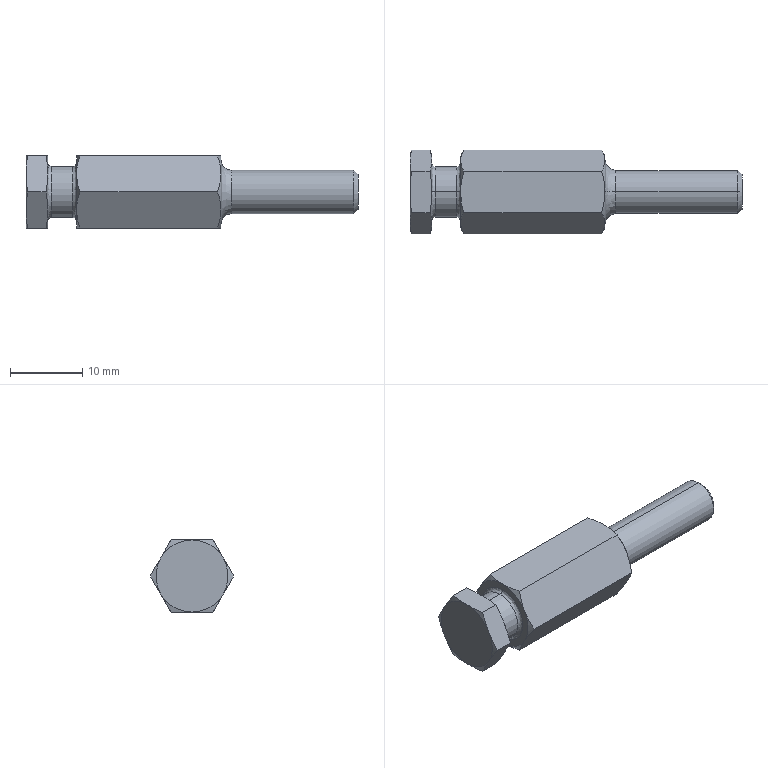Part | STEP file | fjdl6_1_0_4_20_2_03 | 1 solid | 53 faces | box 46 x 11.547 x 10 mm | volume 2689 mm3 | cone 26 | plane 17 | spline 6 | cylinder 4 | commonest cylinder face diameters 6 x2 7 x2